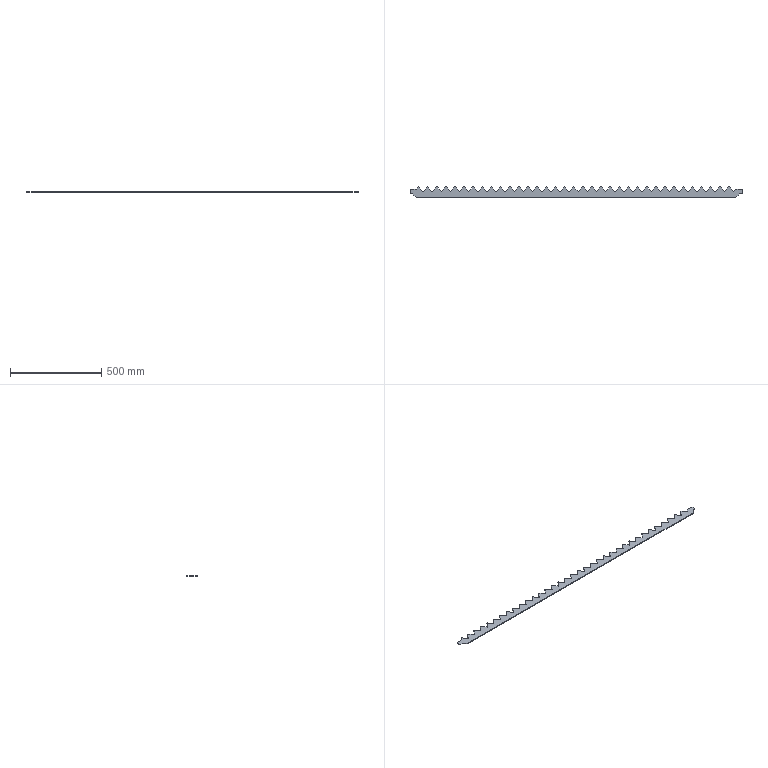Part | SolidWorks | features Fillet 2, Chamfer 1, FlatPattern 1, SMBaseFlange 1, SheetMetal 1 | 1 solid | 156 faces | box 1818 x 58.876 x 4.5 mm | volume 363940 mm3 | plane 82 | cylinder 74 | commonest cylinder face diameters 4 x74